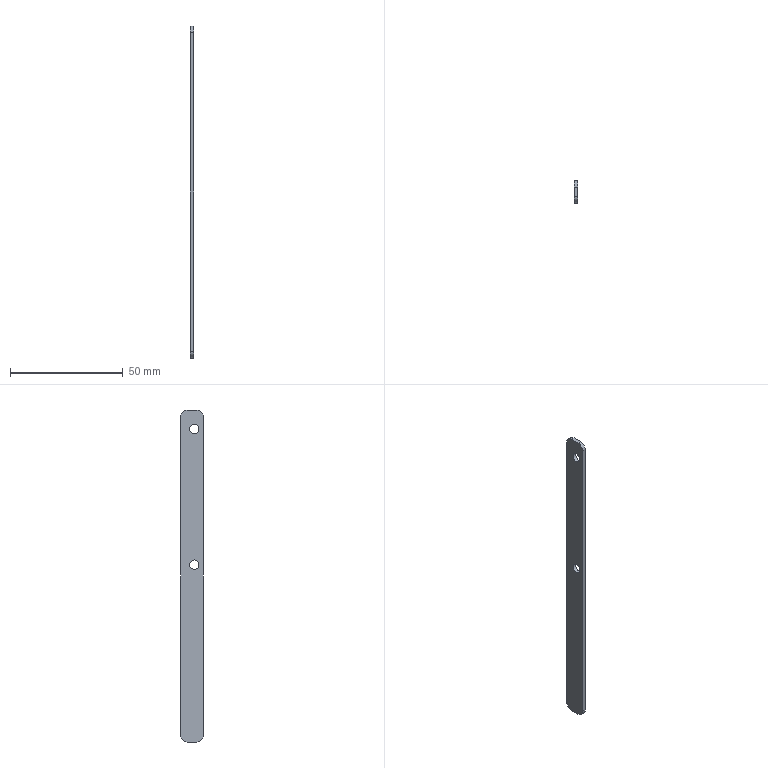Part | NX | features BREP 1 | 1 solid | 12 faces | box 1.5 x 10 x 147 mm | volume 2152 mm3 | cylinder 6 | plane 6 | commonest cylinder face diameters 6 x4 4.2 x2
STEP:
#1=CARTESIAN_POINT('',(1.5,-1.,62.9));
#2=VERTEX_POINT('',#1);
#3=CARTESIAN_POINT('',(1.5,-1.,65.));
#4=DIRECTION('',(1.,0.,0.));
#5=DIRECTION('',(0.,0.,-1.));
#6=AXIS2_PLACEMENT_3D('',#3,#4,#5);
#7=CIRCLE('',#6,2.1);
#8=EDGE_CURVE('',#2,#2,#7,.T.);
#9=ORIENTED_EDGE('',*,*,#8,.T.);
#10=EDGE_LOOP('',(#9));
#11=FACE_BOUND('',#10,.T.);
#12=CARTESIAN_POINT('',(0.,-1.,62.9));
#13=VERTEX_POINT('',#12);
#14=CARTESIAN_POINT('',(0.,-1.,65.));
#15=DIRECTION('',(1.,0.,0.));
#16=DIRECTION('',(0.,0.,-1.));
#17=AXIS2_PLACEMENT_3D('',#14,#15,#16);
#18=CIRCLE('',#17,2.1);
#19=EDGE_CURVE('',#13,#13,#18,.T.);
#20=ORIENTED_EDGE('',*,*,#19,.F.);
#21=EDGE_LOOP('',(#20));
#22=FACE_BOUND('',#21,.T.);
#23=CARTESIAN_POINT('',(1.5,-1.,65.));
#24=DIRECTION('',(1.,0.,0.));
#25=DIRECTION('',(0.,0.,-1.));
#26=AXIS2_PLACEMENT_3D('',#23,#24,#25);
#27=CYLINDRICAL_SURFACE('',#26,2.1);
#28=ADVANCED_FACE('',(#11,#22),#27,.F.);
#29=CARTESIAN_POINT('',(1.5,-1.,2.9));
#30=VERTEX_POINT('',#29);
#31=CARTESIAN_POINT('',(1.5,-1.,5.));
#32=DIRECTION('',(1.,0.,0.));
#33=DIRECTION('',(0.,0.,-1.));
#34=AXIS2_PLACEMENT_3D('',#31,#32,#33);
#35=CIRCLE('',#34,2.1);
#36=EDGE_CURVE('',#30,#30,#35,.T.);
#37=ORIENTED_EDGE('',*,*,#36,.T.);
#38=EDGE_LOOP('',(#37));
#39=FACE_BOUND('',#38,.T.);
#40=CARTESIAN_POINT('',(0.,-1.,2.9));
#41=VERTEX_POINT('',#40);
#42=CARTESIAN_POINT('',(0.,-1.,5.));
#43=DIRECTION('',(1.,0.,0.));
#44=DIRECTION('',(0.,0.,-1.));
#45=AXIS2_PLACEMENT_3D('',#42,#43,#44);
#46=CIRCLE('',#45,2.1);
#47=EDGE_CURVE('',#41,#41,#46,.T.);
#48=ORIENTED_EDGE('',*,*,#47,.F.);
#49=EDGE_LOOP('',(#48));
#50=FACE_BOUND('',#49,.T.);
#51=CARTESIAN_POINT('',(1.5,-1.,5.));
#52=DIRECTION('',(1.,0.,0.));
#53=DIRECTION('',(0.,0.,-1.));
#54=AXIS2_PLACEMENT_3D('',#51,#52,#53);
#55=CYLINDRICAL_SURFACE('',#54,2.1);
#56=ADVANCED_FACE('',(#39,#50),#55,.F.);
#57=CARTESIAN_POINT('',(0.,-2.,-73.5));
#58=VERTEX_POINT('',#57);
#59=CARTESIAN_POINT('',(0.,2.,-73.5));
#60=VERTEX_POINT('',#59);
#61=CARTESIAN_POINT('',(0.,5.,-73.5));
#62=DIRECTION('',(0.,1.,0.));
#63=VECTOR('',#62,1000.);
#64=LINE('',#61,#63);
#65=EDGE_CURVE('',#58,#60,#64,.T.);
#66=ORIENTED_EDGE('',*,*,#65,.T.);
#67=CARTESIAN_POINT('',(1.5,2.,-73.5));
#68=VERTEX_POINT('',#67);
#69=CARTESIAN_POINT('',(1.5,2.,-73.5));
#70=DIRECTION('',(1.,0.,0.));
#71=VECTOR('',#70,1000.);
#72=LINE('',#69,#71);
#73=EDGE_CURVE('',#60,#68,#72,.T.);
#74=ORIENTED_EDGE('',*,*,#73,.T.);
#75=CARTESIAN_POINT('',(1.5,-2.,-73.5));
#76=VERTEX_POINT('',#75);
#77=CARTESIAN_POINT('',(1.5,5.,-73.5));
#78=DIRECTION('',(0.,1.,0.));
#79=VECTOR('',#78,1000.);
#80=LINE('',#77,#79);
#81=EDGE_CURVE('',#76,#68,#80,.T.);
#82=ORIENTED_EDGE('',*,*,#81,.F.);
#83=CARTESIAN_POINT('',(1.5,-2.,-73.5));
#84=DIRECTION('',(-1.,0.,0.));
#85=VECTOR('',#84,1000.);
#86=LINE('',#83,#85);
#87=EDGE_CURVE('',#76,#58,#86,.T.);
#88=ORIENTED_EDGE('',*,*,#87,.T.);
#89=EDGE_LOOP('',(#66,#74,#82,#88));
#90=FACE_BOUND('',#89,.T.);
#91=CARTESIAN_POINT('',(1.5,5.,-73.5));
#92=DIRECTION('',(0.,0.,1.));
#93=DIRECTION('',(1.,0.,0.));
#94=AXIS2_PLACEMENT_3D('',#91,#92,#93);
#95=PLANE('',#94);
#96=ADVANCED_FACE('',(#90),#95,.F.);
#97=CARTESIAN_POINT('',(1.5,5.,-70.5));
#98=VERTEX_POINT('',#97);
#99=CARTESIAN_POINT('',(1.5,5.,70.5));
#100=VERTEX_POINT('',#99);
#101=CARTESIAN_POINT('',(1.5,5.,73.5));
#102=DIRECTION('',(0.,0.,1.));
#103=VECTOR('',#102,1000.);
#104=LINE('',#101,#103);
#105=EDGE_CURVE('',#98,#100,#104,.T.);
#106=ORIENTED_EDGE('',*,*,#105,.F.);
#107=CARTESIAN_POINT('',(0.,5.,-70.5));
#108=VERTEX_POINT('',#107);
#109=CARTESIAN_POINT('',(1.5,5.,-70.5));
#110=DIRECTION('',(-1.,0.,0.));
#111=VECTOR('',#110,1000.);
#112=LINE('',#109,#111);
#113=EDGE_CURVE('',#98,#108,#112,.T.);
#114=ORIENTED_EDGE('',*,*,#113,.T.);
#115=CARTESIAN_POINT('',(0.,5.,70.5));
#116=VERTEX_POINT('',#115);
#117=CARTESIAN_POINT('',(0.,5.,73.5));
#118=DIRECTION('',(0.,0.,1.));
#119=VECTOR('',#118,1000.);
#120=LINE('',#117,#119);
#121=EDGE_CURVE('',#108,#116,#120,.T.);
#122=ORIENTED_EDGE('',*,*,#121,.T.);
#123=CARTESIAN_POINT('',(1.5,5.,70.5));
#124=DIRECTION('',(1.,0.,0.));
#125=VECTOR('',#124,1000.);
#126=LINE('',#123,#125);
#127=EDGE_CURVE('',#116,#100,#126,.T.);
#128=ORIENTED_EDGE('',*,*,#127,.T.);
#129=EDGE_LOOP('',(#106,#114,#122,#128));
#130=FACE_BOUND('',#129,.T.);
#131=CARTESIAN_POINT('',(1.5,5.,73.5));
#132=DIRECTION('',(0.,-1.,0.));
#133=DIRECTION('',(0.,0.,-1.));
#134=AXIS2_PLACEMENT_3D('',#131,#132,#133);
#135=PLANE('',#134);
#136=ADVANCED_FACE('',(#130),#135,.F.);
#137=CARTESIAN_POINT('',(1.5,2.,73.5));
#138=VERTEX_POINT('',#137);
#139=CARTESIAN_POINT('',(1.5,-2.,73.5));
#140=VERTEX_POINT('',#139);
#141=CARTESIAN_POINT('',(1.5,5.,73.5));
#142=DIRECTION('',(0.,-1.,0.));
#143=VECTOR('',#142,1000.);
#144=LINE('',#141,#143);
#145=EDGE_CURVE('',#138,#140,#144,.T.);
#146=ORIENTED_EDGE('',*,*,#145,.F.);
#147=CARTESIAN_POINT('',(0.,2.,73.5));
#148=VERTEX_POINT('',#147);
#149=CARTESIAN_POINT('',(1.5,2.,73.5));
#150=DIRECTION('',(-1.,0.,0.));
#151=VECTOR('',#150,1000.);
#152=LINE('',#149,#151);
#153=EDGE_CURVE('',#138,#148,#152,.T.);
#154=ORIENTED_EDGE('',*,*,#153,.T.);
#155=CARTESIAN_POINT('',(0.,-2.,73.5));
#156=VERTEX_POINT('',#155);
#157=CARTESIAN_POINT('',(0.,5.,73.5));
#158=DIRECTION('',(0.,-1.,0.));
#159=VECTOR('',#158,1000.);
#160=LINE('',#157,#159);
#161=EDGE_CURVE('',#148,#156,#160,.T.);
#162=ORIENTED_EDGE('',*,*,#161,.T.);
#163=CARTESIAN_POINT('',(1.5,-2.,73.5));
#164=DIRECTION('',(1.,0.,0.));
#165=VECTOR('',#164,1000.);
#166=LINE('',#163,#165);
#167=EDGE_CURVE('',#156,#140,#166,.T.);
#168=ORIENTED_EDGE('',*,*,#167,.T.);
#169=EDGE_LOOP('',(#146,#154,#162,#168));
#170=FACE_BOUND('',#169,.T.);
#171=CARTESIAN_POINT('',(1.5,5.,73.5));
#172=DIRECTION('',(0.,0.,-1.));
#173=DIRECTION('',(-1.,0.,0.));
#174=AXIS2_PLACEMENT_3D('',#171,#172,#173);
#175=PLANE('',#174);
#176=ADVANCED_FACE('',(#170),#175,.F.);
#177=CARTESIAN_POINT('',(0.,-5.,70.5));
#178=VERTEX_POINT('',#177);
#179=CARTESIAN_POINT('',(0.,-5.,-70.5));
#180=VERTEX_POINT('',#179);
#181=CARTESIAN_POINT('',(0.,-5.,73.5));
#182=DIRECTION('',(0.,0.,-1.));
#183=VECTOR('',#182,1000.);
#184=LINE('',#181,#183);
#185=EDGE_CURVE('',#178,#180,#184,.T.);
#186=ORIENTED_EDGE('',*,*,#185,.T.);
#187=CARTESIAN_POINT('',(1.5,-5.,-70.5));
#188=VERTEX_POINT('',#187);
#189=CARTESIAN_POINT('',(1.5,-5.,-70.5));
#190=DIRECTION('',(1.,0.,0.));
#191=VECTOR('',#190,1000.);
#192=LINE('',#189,#191);
#193=EDGE_CURVE('',#180,#188,#192,.T.);
#194=ORIENTED_EDGE('',*,*,#193,.T.);
#195=CARTESIAN_POINT('',(1.5,-5.,70.5));
#196=VERTEX_POINT('',#195);
#197=CARTESIAN_POINT('',(1.5,-5.,73.5));
#198=DIRECTION('',(0.,0.,-1.));
#199=VECTOR('',#198,1000.);
#200=LINE('',#197,#199);
#201=EDGE_CURVE('',#196,#188,#200,.T.);
#202=ORIENTED_EDGE('',*,*,#201,.F.);
#203=CARTESIAN_POINT('',(1.5,-5.,70.5));
#204=DIRECTION('',(-1.,0.,0.));
#205=VECTOR('',#204,1000.);
#206=LINE('',#203,#205);
#207=EDGE_CURVE('',#196,#178,#206,.T.);
#208=ORIENTED_EDGE('',*,*,#207,.T.);
#209=EDGE_LOOP('',(#186,#194,#202,#208));
#210=FACE_BOUND('',#209,.T.);
#211=CARTESIAN_POINT('',(1.5,-5.,73.5));
#212=DIRECTION('',(0.,1.,0.));
#213=DIRECTION('',(0.,0.,1.));
#214=AXIS2_PLACEMENT_3D('',#211,#212,#213);
#215=PLANE('',#214);
#216=ADVANCED_FACE('',(#210),#215,.F.);
#217=ORIENTED_EDGE('',*,*,#8,.F.);
#218=EDGE_LOOP('',(#217));
#219=FACE_BOUND('',#218,.T.);
#220=ORIENTED_EDGE('',*,*,#36,.F.);
#221=EDGE_LOOP('',(#220));
#222=FACE_BOUND('',#221,.T.);
#223=ORIENTED_EDGE('',*,*,#81,.T.);
#224=CARTESIAN_POINT('',(1.5,2.,-70.5));
#225=DIRECTION('',(1.,0.,0.));
#226=DIRECTION('',(0.,0.,-1.));
#227=AXIS2_PLACEMENT_3D('',#224,#225,#226);
#228=CIRCLE('',#227,3.);
#229=EDGE_CURVE('',#68,#98,#228,.T.);
#230=ORIENTED_EDGE('',*,*,#229,.T.);
#231=ORIENTED_EDGE('',*,*,#105,.T.);
#232=CARTESIAN_POINT('',(1.5,2.,70.5));
#233=DIRECTION('',(1.,0.,0.));
#234=DIRECTION('',(0.,0.,-1.));
#235=AXIS2_PLACEMENT_3D('',#232,#233,#234);
#236=CIRCLE('',#235,3.);
#237=EDGE_CURVE('',#100,#138,#236,.T.);
#238=ORIENTED_EDGE('',*,*,#237,.T.);
#239=ORIENTED_EDGE('',*,*,#145,.T.);
#240=CARTESIAN_POINT('',(1.5,-2.,70.5));
#241=DIRECTION('',(1.,0.,0.));
#242=DIRECTION('',(0.,0.,-1.));
#243=AXIS2_PLACEMENT_3D('',#240,#241,#242);
#244=CIRCLE('',#243,3.);
#245=EDGE_CURVE('',#140,#196,#244,.T.);
#246=ORIENTED_EDGE('',*,*,#245,.T.);
#247=ORIENTED_EDGE('',*,*,#201,.T.);
#248=CARTESIAN_POINT('',(1.5,-2.,-70.5));
#249=DIRECTION('',(1.,0.,0.));
#250=DIRECTION('',(0.,0.,-1.));
#251=AXIS2_PLACEMENT_3D('',#248,#249,#250);
#252=CIRCLE('',#251,3.);
#253=EDGE_CURVE('',#188,#76,#252,.T.);
#254=ORIENTED_EDGE('',*,*,#253,.T.);
#255=EDGE_LOOP('',(#223,#230,#231,#238,#239,#246,#247,#254));
#256=FACE_BOUND('',#255,.T.);
#257=CARTESIAN_POINT('',(1.5,0.,0.));
#258=DIRECTION('',(1.,0.,0.));
#259=DIRECTION('',(0.,0.,-1.));
#260=AXIS2_PLACEMENT_3D('',#257,#258,#259);
#261=PLANE('',#260);
#262=ADVANCED_FACE('',(#219,#222,#256),#261,.T.);
#263=ORIENTED_EDGE('',*,*,#19,.T.);
#264=EDGE_LOOP('',(#263));
#265=FACE_BOUND('',#264,.T.);
#266=ORIENTED_EDGE('',*,*,#47,.T.);
#267=EDGE_LOOP('',(#266));
#268=FACE_BOUND('',#267,.T.);
#269=ORIENTED_EDGE('',*,*,#121,.F.);
#270=CARTESIAN_POINT('',(0.,2.,-70.5));
#271=DIRECTION('',(-1.,0.,0.));
#272=DIRECTION('',(0.,0.,-1.));
#273=AXIS2_PLACEMENT_3D('',#270,#271,#272);
#274=CIRCLE('',#273,3.);
#275=EDGE_CURVE('',#108,#60,#274,.T.);
#276=ORIENTED_EDGE('',*,*,#275,.T.);
#277=ORIENTED_EDGE('',*,*,#65,.F.);
#278=CARTESIAN_POINT('',(0.,-2.,-70.5));
#279=DIRECTION('',(-1.,0.,0.));
#280=DIRECTION('',(0.,0.,-1.));
#281=AXIS2_PLACEMENT_3D('',#278,#279,#280);
#282=CIRCLE('',#281,3.);
#283=EDGE_CURVE('',#58,#180,#282,.T.);
#284=ORIENTED_EDGE('',*,*,#283,.T.);
#285=ORIENTED_EDGE('',*,*,#185,.F.);
#286=CARTESIAN_POINT('',(0.,-2.,70.5));
#287=DIRECTION('',(-1.,0.,0.));
#288=DIRECTION('',(0.,0.,-1.));
#289=AXIS2_PLACEMENT_3D('',#286,#287,#288);
#290=CIRCLE('',#289,3.);
#291=EDGE_CURVE('',#178,#156,#290,.T.);
#292=ORIENTED_EDGE('',*,*,#291,.T.);
#293=ORIENTED_EDGE('',*,*,#161,.F.);
#294=CARTESIAN_POINT('',(0.,2.,70.5));
#295=DIRECTION('',(-1.,0.,0.));
#296=DIRECTION('',(0.,0.,-1.));
#297=AXIS2_PLACEMENT_3D('',#294,#295,#296);
#298=CIRCLE('',#297,3.);
#299=EDGE_CURVE('',#148,#116,#298,.T.);
#300=ORIENTED_EDGE('',*,*,#299,.T.);
#301=EDGE_LOOP('',(#269,#276,#277,#284,#285,#292,#293,#300));
#302=FACE_BOUND('',#301,.T.);
#303=CARTESIAN_POINT('',(0.,0.,0.));
#304=DIRECTION('',(1.,0.,0.));
#305=DIRECTION('',(0.,0.,-1.));
#306=AXIS2_PLACEMENT_3D('',#303,#304,#305);
#307=PLANE('',#306);
#308=ADVANCED_FACE('',(#265,#268,#302),#307,.F.);
#309=ORIENTED_EDGE('',*,*,#229,.F.);
#310=ORIENTED_EDGE('',*,*,#73,.F.);
#311=ORIENTED_EDGE('',*,*,#275,.F.);
#312=ORIENTED_EDGE('',*,*,#113,.F.);
#313=EDGE_LOOP('',(#309,#310,#311,#312));
#314=FACE_BOUND('',#313,.T.);
#315=CARTESIAN_POINT('',(1.5,2.,-70.5));
#316=DIRECTION('',(-1.,0.,0.));
#317=DIRECTION('',(0.,0.,1.));
#318=AXIS2_PLACEMENT_3D('',#315,#316,#317);
#319=CYLINDRICAL_SURFACE('',#318,3.);
#320=ADVANCED_FACE('',(#314),#319,.T.);
#321=ORIENTED_EDGE('',*,*,#237,.F.);
#322=ORIENTED_EDGE('',*,*,#127,.F.);
#323=ORIENTED_EDGE('',*,*,#299,.F.);
#324=ORIENTED_EDGE('',*,*,#153,.F.);
#325=EDGE_LOOP('',(#321,#322,#323,#324));
#326=FACE_BOUND('',#325,.T.);
#327=CARTESIAN_POINT('',(1.5,2.,70.5));
#328=DIRECTION('',(-1.,0.,0.));
#329=DIRECTION('',(0.,0.,1.));
#330=AXIS2_PLACEMENT_3D('',#327,#328,#329);
#331=CYLINDRICAL_SURFACE('',#330,3.);
#332=ADVANCED_FACE('',(#326),#331,.T.);
#333=ORIENTED_EDGE('',*,*,#253,.F.);
#334=ORIENTED_EDGE('',*,*,#193,.F.);
#335=ORIENTED_EDGE('',*,*,#283,.F.);
#336=ORIENTED_EDGE('',*,*,#87,.F.);
#337=EDGE_LOOP('',(#333,#334,#335,#336));
#338=FACE_BOUND('',#337,.T.);
#339=CARTESIAN_POINT('',(1.5,-2.,-70.5));
#340=DIRECTION('',(-1.,0.,0.));
#341=DIRECTION('',(0.,0.,1.));
#342=AXIS2_PLACEMENT_3D('',#339,#340,#341);
#343=CYLINDRICAL_SURFACE('',#342,3.);
#344=ADVANCED_FACE('',(#338),#343,.T.);
#345=ORIENTED_EDGE('',*,*,#245,.F.);
#346=ORIENTED_EDGE('',*,*,#167,.F.);
#347=ORIENTED_EDGE('',*,*,#291,.F.);
#348=ORIENTED_EDGE('',*,*,#207,.F.);
#349=EDGE_LOOP('',(#345,#346,#347,#348));
#350=FACE_BOUND('',#349,.T.);
#351=CARTESIAN_POINT('',(1.5,-2.,70.5));
#352=DIRECTION('',(-1.,0.,0.));
#353=DIRECTION('',(0.,0.,1.));
#354=AXIS2_PLACEMENT_3D('',#351,#352,#353);
#355=CYLINDRICAL_SURFACE('',#354,3.);
#356=ADVANCED_FACE('',(#350),#355,.T.);
#357=CLOSED_SHELL('',(#28,#56,#96,#136,#176,#216,#262,#308,#320,#332,#344,#356));
#358=MANIFOLD_SOLID_BREP('',#357);
#359=(LENGTH_UNIT()NAMED_UNIT(*)SI_UNIT(.MILLI.,.METRE.));
#360=UNCERTAINTY_MEASURE_WITH_UNIT(LENGTH_MEASURE(0.00001),#359,'','');
#361=(NAMED_UNIT(*)PLANE_ANGLE_UNIT()SI_UNIT($,.RADIAN.));
#362=(NAMED_UNIT(*)SI_UNIT($,.STERADIAN.)SOLID_ANGLE_UNIT());
#363=(GEOMETRIC_REPRESENTATION_CONTEXT(3)GLOBAL_UNCERTAINTY_ASSIGNED_CONTEXT((#360))GLOBAL_UNIT_ASSIGNED_CONTEXT((#359,#361,#362))REPRESENTATION_CONTEXT('',''));
#364=ADVANCED_BREP_SHAPE_REPRESENTATION('',(#358),#363);